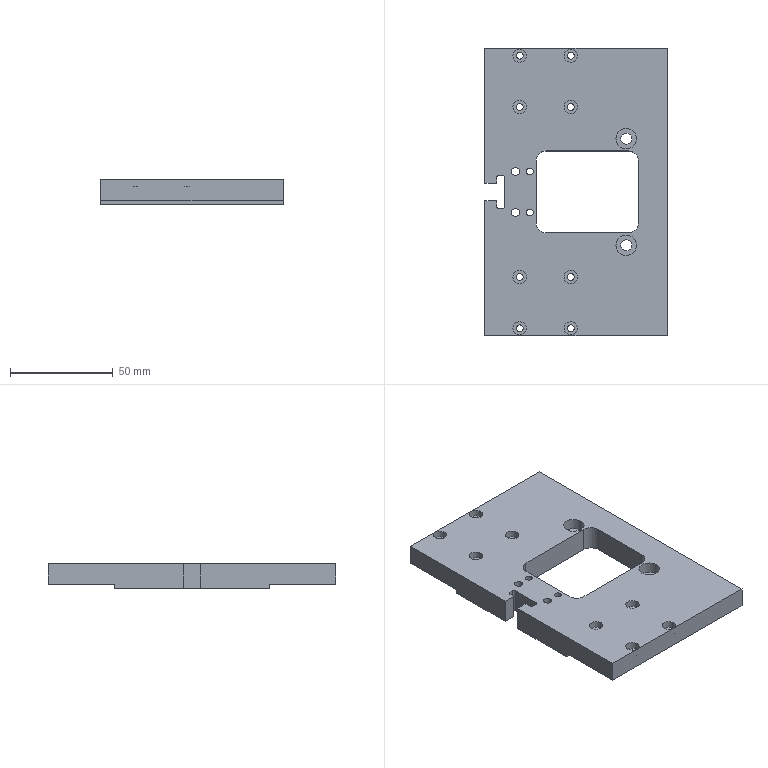CAM job | NX | 3-axis milling, drilling | part box 89 x 140 x 12 mm | stock box 94 x 145 x 15 mm
Tools:
number,name,description,diameter,corner_radius,flute_length,length,flutes
4,D4,平底铣刀-粗,4.0,0.0,25.0,75.0,2
6,D6,平底铣刀-粗,6.0,0.0,25.0,75.0,2
9,D10,平底铣刀-粗,10.0,0.0,35.0,75.0,2
19,D2-J,平底铣刀-精,2.0,0.0,50.0,75.0,2
11,D4-J,平底铣刀-精,4.0,0.0,50.0,75.0,2
7,D6-J,平底铣刀-精,6.0,0.0,25.0,75.0,2
10,D10-J,平底铣刀-精,10.0,0.0,35.0,75.0,2
1,D80R0.8_FLYCUTTER,圆鼻刀-粗,80.0,0.8,50.0,75.0,2
1,D80R0.8_FLYCUTTER-J,圆鼻刀-精,80.0,0.8,50.0,75.0,2
2,D6_CHAMFER,倒角刀,6.0,0.0,3.0,25.0,2
21,M4X0.7,丝锥,3.3,0.0,35.0,50.0,2
23,D4_REAMER,Drilling Tool,4.0,0.0,75.0,100.0,6
13,ZT3.4,钻头,3.4,0.0,35.0,50.0,2
18,ZT5.5,钻头,5.5,0.0,35.0,50.0,2
17,ZT3.9,Drilling Tool,3.9,0.0,35.0,50.0,2
Operations:
program,operation,operation_type,tool,method,geometry_group,spindle_rpm,surface_speed,feed_per_tooth,feed_cut,feed_plunge,cut_length_mm,path_length_mm,cut_time_min,machine_time_min
B,FLOORWALL_FLYFACE_ROUGH_COPY,VolumeBased25DMillingOperation,D80R0.8_FLYCUTTER,LAYERED_ROUGH-DEPTHK-STEPG,W-B,2800.0,703.696,0.5357,3000.0,100.0,2478.487,2707.714,0.8262,0.8491
B,FLOORWALL_FLYFACE_FINISH_COPY,VolumeBased25DMillingOperation,D80R0.8_FLYCUTTER-J,SIDEWALL_FINISH-DEPTHK-STEPG,W-B,4000.0,1005.28,0.125,1000.0,100.0,495.11,591.11,0.4951,0.5047
B,FLOORWALL_LAYERED_ROUGH-MID_COPY,VolumeBased25DMillingOperation,D10,LAYERED_ROUGH-DEPTHK-STEPG,W-B,8000.0,251.32,0.25,4000.0,100.0,4248.61,5050.353,1.062,1.142
B,NG_DRILLCHAMFER_3,Operation,D6_CHAMFER,METHOD,W-B,8000.0,150.796,0.0625,1000.0,0.0,10.4,144.024,0.0104,0.0238
B,NG_DRILLCHAMFER_4,Operation,D6_CHAMFER,METHOD,W-B,8000.0,150.796,0.0625,1000.0,0.0,40.0,439.13,0.04,0.0799
B,NG_DRILLCHAMFER_5,Operation,D6_CHAMFER,METHOD,W-B,8000.0,150.796,0.0625,1000.0,0.0,10.6,144.424,0.0106,0.024
B,MILL_CHAMFER_3,PlanarMilling,D6_CHAMFER,METHOD,W-B,8000.0,150.796,0.075,1200.0,100.0,35.589,292.483,0.0297,0.0553
B,PLANARDEBURR_6X45L_COPY,SurfaceContour,D6_CHAMFER,CLIMB_CHAMFER-DEPTH0-STEPG,W-B,6500.0,122.519,0.1154,1500.0,100.0,972.829,1998.517,0.6486,0.7511
B,FLOORWALL_FINISH_BOTTOM-MID_COPY,VolumeBased25DMillingOperation,D10-J,FINISH_STEPDEPTH_OFF,W-B,8000.0,251.32,0.0625,1000.0,100.0,1220.576,1412.704,1.221,1.24
B,FLOORWALL_FINISH_SIDE-MID-SELBOTTOM_COPY,VolumeBased25DMillingOperation,D10-J,SIDEWALL_FINISH-DEPTHK-STEPG,W-B,8000.0,251.32,0.0625,1000.0,100.0,215.363,340.761,0.2154,0.2279
A,FACEMILL_TOP,FaceMilling,D80R0.8_FLYCUTTER,SIDEWALL_FINISH-DEPTHK-STEPG,W-A,4500.0,1385.0,0.1667,1500.0,100.0,758.5,854.5,0.5057,0.5153
A,SPOTDRILL_DEPTH0.8,Operation,D6_CHAMFER,NONE,W-A,8000.0,150.796,0.0312,500.0,90.0,25.2,473.143,0.0504,0.0952
A,THRUHOLE_M4_TAPDRILL,Operation,ZT3.4,NONE,W-A,3000.0,31.102,0.05,300.0,90.0,38.0,197.025,0.1267,0.1426
A,COUNTERBORE_DRILL_SEG0,Operation,ZT3.4,NONE,W-A,2800.0,29.908,0.0179,100.0,90.0,112.172,564.469,1.122,1.167
A,THRUHOLE_FINE4.0_PREDRILL,Operation,ZT3.9,NONE,W-A,3000.0,36.757,0.0417,250.0,90.0,34.252,189.528,0.137,0.1525
A,COUNTERBORE_DRILL_SEG0_2,Operation,ZT5.5,NONE,W-A,1200.0,20.735,0.0625,150.0,90.0,33.305,219.619,0.222,0.2407
A,THRUSLOT_ROUGH_1,VolumeBased25DMillingOperation,D10,METHOD,W-A,9000.0,169.646,0.0667,1200.0,100.0,5987.113,6097.513,4.989,5
A,OUTLINE_ROUGH_2,VolumeBased25DMillingOperation,D10,METHOD,W-A,8000.0,251.327,0.375,6000.0,80.0,8358.58,8469.08,1.393,1.404
A,HOLEMILL_ROUGH_D6_1,CylinderMilling,D6,NONE,W-A,8000.0,150.796,0.075,1200.0,100.0,317.799,579.599,0.2648,0.291
A,HOLEMILL_ROUGH_D4_1,CylinderMilling,D4,NONE,W-A,8000.0,100.531,0.075,1200.0,100.0,838.824,1895.024,0.699,0.8046
A,HOLEMILL_FINISH_D6_1,CylinderMilling,D6-J,FINISH_STEPDEPTH_OFF,W-A,8000.0,150.796,0.0312,500.0,100.0,66.797,329.597,0.1336,0.1599
A,HOLEMILL_FINISH_D4_1,CylinderMilling,D4-J,FINISH_STEPDEPTH_OFF,W-A,8000.0,100.531,0.0312,500.0,100.0,151.649,1207.849,0.3033,0.4089
A,SLOT_FINISH_1,VolumeBased25DMillingOperation,D6-J,METHOD,W-A,9000.0,169.646,0.0333,600.0,100.0,309.589,446.189,0.516,0.5296
A,ZLEVEL_SMOOTH_CORNER_D6_REF12_COPY,ZLevelMilling,D6-J,LAYERED_FINISH-DEPTHK-STEPG,W-A,8000.0,150.796,0.125,2000.0,100.0,1268.179,1379.229,0.6341,0.6452
A,ZLEVEL_SMOOTH_CORNER_D2_REF6_COPY,ZLevelMilling,D2-J,LAYERED_FINISH-DEPTHK-STEPG,W-A,8000.0,50.266,0.0938,1500.0,100.0,2452.557,2584.367,1.635,1.648
A,SELBODY_ONLY,SurfaceContour,D6_CHAMFER,METHOD,W-A,8000.0,150.796,0.1875,3000.0,100.0,680.077,916.394,0.2267,0.2503
A,NG_DRILLCHAMFER_1,Operation,D6_CHAMFER,METHOD,W-A,8000.0,150.796,0.0312,500.0,0.0,10.4,144.024,0.0208,0.0342
A,NG_DRILLCHAMFER_2,Operation,D6_CHAMFER,METHOD,W-A,8000.0,150.796,0.0312,500.0,0.0,10.6,144.424,0.0212,0.0346
A,MILL_CHAMFER_1,PlanarMilling,D6_CHAMFER,NONE,W-A,8000.0,150.796,0.0312,500.0,100.0,234.043,1233.113,0.4681,0.568
A,MILL_CHAMFER_2,PlanarMilling,D6_CHAMFER,NONE,W-A,8000.0,150.796,0.05,800.0,100.0,80.502,321.113,0.1006,0.1247
A,REAM,Operation,D4_REAMER,METHOD,W-A,500.0,6.283,0.0167,50.0,0.0,28.0,177.025,0.56,0.5749
A,THRUHOLE_TAPM4,Operation,M4X0.7,METHOD,W-A,600.0,6.22,0.0006,0.7,90.0,32.0,185.025,45.714,45.73
A,OUTLINE_SEMIFINISH_2,VolumeBased25DMillingOperation,D6-J,METHOD,W-A,9000.0,169.646,0.0667,1200.0,100.0,499.173,622.173,0.416,0.4283